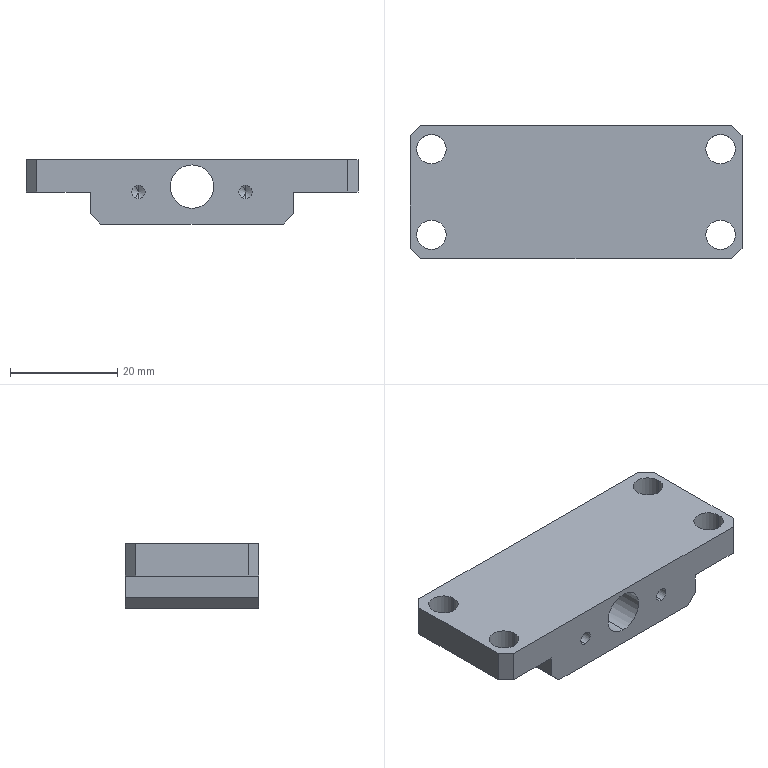Part | STEP file | 11-FG-SZ03111 | 1 solid | 38 faces | box 62 x 25 x 12 mm | volume 12866 mm3 | cylinder 18 | plane 16 | cone 4 | commonest cylinder face diameters 5.5 x8 2.5 x4 3.3 x4 8.1 x2
STEP:
#1=CARTESIAN_POINT('',(-29.75,8.,12.));
#2=VERTEX_POINT('',#1);
#3=CARTESIAN_POINT('',(-24.25,8.,12.));
#4=VERTEX_POINT('',#3);
#5=CARTESIAN_POINT('',(-27.,8.,12.));
#6=DIRECTION('',(0.,0.,1.));
#7=DIRECTION('',(1.,0.,0.));
#8=AXIS2_PLACEMENT_3D('',#5,#6,#7);
#9=CIRCLE('',#8,2.75);
#10=EDGE_CURVE('',#2,#4,#9,.T.);
#11=ORIENTED_EDGE('',*,*,#10,.T.);
#12=CARTESIAN_POINT('',(-24.25,8.,6.));
#13=VERTEX_POINT('',#12);
#14=CARTESIAN_POINT('',(-24.25,8.,24.));
#15=DIRECTION('',(0.,0.,-1.));
#16=VECTOR('',#15,1000.);
#17=LINE('',#14,#16);
#18=EDGE_CURVE('',#4,#13,#17,.T.);
#19=ORIENTED_EDGE('',*,*,#18,.T.);
#20=CARTESIAN_POINT('',(-29.75,8.,6.));
#21=VERTEX_POINT('',#20);
#22=CARTESIAN_POINT('',(-27.,8.,6.));
#23=DIRECTION('',(0.,0.,-1.));
#24=DIRECTION('',(-1.,0.,0.));
#25=AXIS2_PLACEMENT_3D('',#22,#23,#24);
#26=CIRCLE('',#25,2.75);
#27=EDGE_CURVE('',#13,#21,#26,.T.);
#28=ORIENTED_EDGE('',*,*,#27,.T.);
#29=CARTESIAN_POINT('',(-29.75,8.,24.));
#30=DIRECTION('',(0.,0.,-1.));
#31=VECTOR('',#30,1000.);
#32=LINE('',#29,#31);
#33=EDGE_CURVE('',#2,#21,#32,.T.);
#34=ORIENTED_EDGE('',*,*,#33,.F.);
#35=EDGE_LOOP('',(#11,#19,#28,#34));
#36=FACE_OUTER_BOUND('',#35,.T.);
#37=CARTESIAN_POINT('',(-27.,8.,24.));
#38=DIRECTION('',(0.,0.,-1.));
#39=DIRECTION('',(-1.,0.,0.));
#40=AXIS2_PLACEMENT_3D('',#37,#38,#39);
#41=CYLINDRICAL_SURFACE('',#40,2.75);
#42=ADVANCED_FACE('',(#36),#41,.F.);
#43=CARTESIAN_POINT('',(-29.75,-8.,12.));
#44=VERTEX_POINT('',#43);
#45=CARTESIAN_POINT('',(-24.25,-8.,12.));
#46=VERTEX_POINT('',#45);
#47=CARTESIAN_POINT('',(-27.,-8.,12.));
#48=DIRECTION('',(0.,0.,1.));
#49=DIRECTION('',(1.,0.,0.));
#50=AXIS2_PLACEMENT_3D('',#47,#48,#49);
#51=CIRCLE('',#50,2.75);
#52=EDGE_CURVE('',#44,#46,#51,.T.);
#53=ORIENTED_EDGE('',*,*,#52,.T.);
#54=CARTESIAN_POINT('',(-24.25,-8.,6.));
#55=VERTEX_POINT('',#54);
#56=CARTESIAN_POINT('',(-24.25,-8.,24.));
#57=DIRECTION('',(0.,0.,-1.));
#58=VECTOR('',#57,1000.);
#59=LINE('',#56,#58);
#60=EDGE_CURVE('',#46,#55,#59,.T.);
#61=ORIENTED_EDGE('',*,*,#60,.T.);
#62=CARTESIAN_POINT('',(-29.75,-8.,6.));
#63=VERTEX_POINT('',#62);
#64=CARTESIAN_POINT('',(-27.,-8.,6.));
#65=DIRECTION('',(0.,0.,-1.));
#66=DIRECTION('',(-1.,0.,0.));
#67=AXIS2_PLACEMENT_3D('',#64,#65,#66);
#68=CIRCLE('',#67,2.75);
#69=EDGE_CURVE('',#55,#63,#68,.T.);
#70=ORIENTED_EDGE('',*,*,#69,.T.);
#71=CARTESIAN_POINT('',(-29.75,-8.,24.));
#72=DIRECTION('',(0.,0.,-1.));
#73=VECTOR('',#72,1000.);
#74=LINE('',#71,#73);
#75=EDGE_CURVE('',#44,#63,#74,.T.);
#76=ORIENTED_EDGE('',*,*,#75,.F.);
#77=EDGE_LOOP('',(#53,#61,#70,#76));
#78=FACE_OUTER_BOUND('',#77,.T.);
#79=CARTESIAN_POINT('',(-27.,-8.,24.));
#80=DIRECTION('',(0.,0.,-1.));
#81=DIRECTION('',(-1.,0.,0.));
#82=AXIS2_PLACEMENT_3D('',#79,#80,#81);
#83=CYLINDRICAL_SURFACE('',#82,2.75);
#84=ADVANCED_FACE('',(#78),#83,.F.);
#85=CARTESIAN_POINT('',(24.25,-8.,12.));
#86=VERTEX_POINT('',#85);
#87=CARTESIAN_POINT('',(29.75,-8.,12.));
#88=VERTEX_POINT('',#87);
#89=CARTESIAN_POINT('',(27.,-8.,12.));
#90=DIRECTION('',(0.,0.,1.));
#91=DIRECTION('',(1.,0.,0.));
#92=AXIS2_PLACEMENT_3D('',#89,#90,#91);
#93=CIRCLE('',#92,2.75);
#94=EDGE_CURVE('',#86,#88,#93,.T.);
#95=ORIENTED_EDGE('',*,*,#94,.T.);
#96=CARTESIAN_POINT('',(29.75,-8.,6.));
#97=VERTEX_POINT('',#96);
#98=CARTESIAN_POINT('',(29.75,-8.,24.));
#99=DIRECTION('',(0.,0.,-1.));
#100=VECTOR('',#99,1000.);
#101=LINE('',#98,#100);
#102=EDGE_CURVE('',#88,#97,#101,.T.);
#103=ORIENTED_EDGE('',*,*,#102,.T.);
#104=CARTESIAN_POINT('',(24.25,-8.,6.));
#105=VERTEX_POINT('',#104);
#106=CARTESIAN_POINT('',(27.,-8.,6.));
#107=DIRECTION('',(0.,0.,-1.));
#108=DIRECTION('',(-1.,0.,0.));
#109=AXIS2_PLACEMENT_3D('',#106,#107,#108);
#110=CIRCLE('',#109,2.75);
#111=EDGE_CURVE('',#97,#105,#110,.T.);
#112=ORIENTED_EDGE('',*,*,#111,.T.);
#113=CARTESIAN_POINT('',(24.25,-8.,24.));
#114=DIRECTION('',(0.,0.,-1.));
#115=VECTOR('',#114,1000.);
#116=LINE('',#113,#115);
#117=EDGE_CURVE('',#86,#105,#116,.T.);
#118=ORIENTED_EDGE('',*,*,#117,.F.);
#119=EDGE_LOOP('',(#95,#103,#112,#118));
#120=FACE_OUTER_BOUND('',#119,.T.);
#121=CARTESIAN_POINT('',(27.,-8.,24.));
#122=DIRECTION('',(0.,0.,-1.));
#123=DIRECTION('',(-1.,0.,0.));
#124=AXIS2_PLACEMENT_3D('',#121,#122,#123);
#125=CYLINDRICAL_SURFACE('',#124,2.75);
#126=ADVANCED_FACE('',(#120),#125,.F.);
#127=CARTESIAN_POINT('',(24.25,8.,12.));
#128=VERTEX_POINT('',#127);
#129=CARTESIAN_POINT('',(29.75,8.,12.));
#130=VERTEX_POINT('',#129);
#131=CARTESIAN_POINT('',(27.,8.,12.));
#132=DIRECTION('',(0.,0.,1.));
#133=DIRECTION('',(1.,0.,0.));
#134=AXIS2_PLACEMENT_3D('',#131,#132,#133);
#135=CIRCLE('',#134,2.75);
#136=EDGE_CURVE('',#128,#130,#135,.T.);
#137=ORIENTED_EDGE('',*,*,#136,.T.);
#138=CARTESIAN_POINT('',(29.75,8.,6.));
#139=VERTEX_POINT('',#138);
#140=CARTESIAN_POINT('',(29.75,8.,24.));
#141=DIRECTION('',(0.,0.,-1.));
#142=VECTOR('',#141,1000.);
#143=LINE('',#140,#142);
#144=EDGE_CURVE('',#130,#139,#143,.T.);
#145=ORIENTED_EDGE('',*,*,#144,.T.);
#146=CARTESIAN_POINT('',(24.25,8.,6.));
#147=VERTEX_POINT('',#146);
#148=CARTESIAN_POINT('',(27.,8.,6.));
#149=DIRECTION('',(0.,0.,-1.));
#150=DIRECTION('',(-1.,0.,0.));
#151=AXIS2_PLACEMENT_3D('',#148,#149,#150);
#152=CIRCLE('',#151,2.75);
#153=EDGE_CURVE('',#139,#147,#152,.T.);
#154=ORIENTED_EDGE('',*,*,#153,.T.);
#155=CARTESIAN_POINT('',(24.25,8.,24.));
#156=DIRECTION('',(0.,0.,-1.));
#157=VECTOR('',#156,1000.);
#158=LINE('',#155,#157);
#159=EDGE_CURVE('',#128,#147,#158,.T.);
#160=ORIENTED_EDGE('',*,*,#159,.F.);
#161=EDGE_LOOP('',(#137,#145,#154,#160));
#162=FACE_OUTER_BOUND('',#161,.T.);
#163=CARTESIAN_POINT('',(27.,8.,24.));
#164=DIRECTION('',(0.,0.,-1.));
#165=DIRECTION('',(-1.,0.,0.));
#166=AXIS2_PLACEMENT_3D('',#163,#164,#165);
#167=CYLINDRICAL_SURFACE('',#166,2.75);
#168=ADVANCED_FACE('',(#162),#167,.F.);
#169=CARTESIAN_POINT('',(10.,-5.,7.25));
#170=VERTEX_POINT('',#169);
#171=CARTESIAN_POINT('',(10.,-5.,4.75));
#172=VERTEX_POINT('',#171);
#173=CARTESIAN_POINT('',(10.,-5.,6.));
#174=DIRECTION('',(0.,-1.,0.));
#175=DIRECTION('',(0.,0.,-1.));
#176=AXIS2_PLACEMENT_3D('',#173,#174,#175);
#177=CIRCLE('',#176,1.25);
#178=EDGE_CURVE('',#170,#172,#177,.T.);
#179=ORIENTED_EDGE('',*,*,#178,.F.);
#180=CARTESIAN_POINT('',(10.,-12.5,7.25));
#181=VERTEX_POINT('',#180);
#182=CARTESIAN_POINT('',(10.,-12.5,7.25));
#183=DIRECTION('',(0.,-1.,0.));
#184=VECTOR('',#183,1000.);
#185=LINE('',#182,#184);
#186=EDGE_CURVE('',#170,#181,#185,.T.);
#187=ORIENTED_EDGE('',*,*,#186,.T.);
#188=CARTESIAN_POINT('',(10.,-12.5,4.75));
#189=VERTEX_POINT('',#188);
#190=CARTESIAN_POINT('',(10.,-12.5,6.));
#191=DIRECTION('',(0.,-1.,0.));
#192=DIRECTION('',(0.,0.,-1.));
#193=AXIS2_PLACEMENT_3D('',#190,#191,#192);
#194=CIRCLE('',#193,1.25);
#195=EDGE_CURVE('',#181,#189,#194,.T.);
#196=ORIENTED_EDGE('',*,*,#195,.T.);
#197=CARTESIAN_POINT('',(10.,-12.5,4.75));
#198=DIRECTION('',(0.,-1.,0.));
#199=VECTOR('',#198,1000.);
#200=LINE('',#197,#199);
#201=EDGE_CURVE('',#172,#189,#200,.T.);
#202=ORIENTED_EDGE('',*,*,#201,.F.);
#203=EDGE_LOOP('',(#179,#187,#196,#202));
#204=FACE_OUTER_BOUND('',#203,.T.);
#205=CARTESIAN_POINT('',(10.,-12.5,6.));
#206=DIRECTION('',(0.,-1.,0.));
#207=DIRECTION('',(0.,0.,-1.));
#208=AXIS2_PLACEMENT_3D('',#205,#206,#207);
#209=CYLINDRICAL_SURFACE('',#208,1.25);
#210=ADVANCED_FACE('',(#204),#209,.F.);
#211=CARTESIAN_POINT('',(10.,-4.249,6.));
#212=VERTEX_POINT('',#211);
#213=CARTESIAN_POINT('',(10.,-5.,4.75));
#214=DIRECTION('',(0.,-0.515,-0.8572));
#215=VECTOR('',#214,1000.);
#216=LINE('',#213,#215);
#217=EDGE_CURVE('',#212,#172,#216,.T.);
#218=ORIENTED_EDGE('',*,*,#217,.F.);
#219=CARTESIAN_POINT('',(10.,-5.,7.25));
#220=DIRECTION('',(0.,-0.515,0.8572));
#221=VECTOR('',#220,1000.);
#222=LINE('',#219,#221);
#223=EDGE_CURVE('',#212,#170,#222,.T.);
#224=ORIENTED_EDGE('',*,*,#223,.T.);
#225=ORIENTED_EDGE('',*,*,#178,.T.);
#226=EDGE_LOOP('',(#218,#224,#225));
#227=FACE_OUTER_BOUND('',#226,.T.);
#228=CARTESIAN_POINT('',(10.,-5.,6.));
#229=DIRECTION('',(0.,-1.,0.));
#230=DIRECTION('',(0.,0.,-1.));
#231=AXIS2_PLACEMENT_3D('',#228,#229,#230);
#232=CONICAL_SURFACE('',#231,1.25,1.03);
#233=ADVANCED_FACE('',(#227),#232,.F.);
#234=CARTESIAN_POINT('',(-10.,-5.,7.25));
#235=VERTEX_POINT('',#234);
#236=CARTESIAN_POINT('',(-10.,-5.,4.75));
#237=VERTEX_POINT('',#236);
#238=CARTESIAN_POINT('',(-10.,-5.,6.));
#239=DIRECTION('',(0.,-1.,0.));
#240=DIRECTION('',(0.,0.,-1.));
#241=AXIS2_PLACEMENT_3D('',#238,#239,#240);
#242=CIRCLE('',#241,1.25);
#243=EDGE_CURVE('',#235,#237,#242,.T.);
#244=ORIENTED_EDGE('',*,*,#243,.F.);
#245=CARTESIAN_POINT('',(-10.,-12.5,7.25));
#246=VERTEX_POINT('',#245);
#247=CARTESIAN_POINT('',(-10.,-12.5,7.25));
#248=DIRECTION('',(0.,-1.,0.));
#249=VECTOR('',#248,1000.);
#250=LINE('',#247,#249);
#251=EDGE_CURVE('',#235,#246,#250,.T.);
#252=ORIENTED_EDGE('',*,*,#251,.T.);
#253=CARTESIAN_POINT('',(-10.,-12.5,4.75));
#254=VERTEX_POINT('',#253);
#255=CARTESIAN_POINT('',(-10.,-12.5,6.));
#256=DIRECTION('',(0.,-1.,0.));
#257=DIRECTION('',(0.,0.,-1.));
#258=AXIS2_PLACEMENT_3D('',#255,#256,#257);
#259=CIRCLE('',#258,1.25);
#260=EDGE_CURVE('',#246,#254,#259,.T.);
#261=ORIENTED_EDGE('',*,*,#260,.T.);
#262=CARTESIAN_POINT('',(-10.,-12.5,4.75));
#263=DIRECTION('',(0.,-1.,0.));
#264=VECTOR('',#263,1000.);
#265=LINE('',#262,#264);
#266=EDGE_CURVE('',#237,#254,#265,.T.);
#267=ORIENTED_EDGE('',*,*,#266,.F.);
#268=EDGE_LOOP('',(#244,#252,#261,#267));
#269=FACE_OUTER_BOUND('',#268,.T.);
#270=CARTESIAN_POINT('',(-10.,-12.5,6.));
#271=DIRECTION('',(0.,-1.,0.));
#272=DIRECTION('',(0.,0.,-1.));
#273=AXIS2_PLACEMENT_3D('',#270,#271,#272);
#274=CYLINDRICAL_SURFACE('',#273,1.25);
#275=ADVANCED_FACE('',(#269),#274,.F.);
#276=CARTESIAN_POINT('',(-10.,-4.249,6.));
#277=VERTEX_POINT('',#276);
#278=CARTESIAN_POINT('',(-10.,-5.,4.75));
#279=DIRECTION('',(0.,-0.515,-0.8572));
#280=VECTOR('',#279,1000.);
#281=LINE('',#278,#280);
#282=EDGE_CURVE('',#277,#237,#281,.T.);
#283=ORIENTED_EDGE('',*,*,#282,.F.);
#284=CARTESIAN_POINT('',(-10.,-5.,7.25));
#285=DIRECTION('',(0.,-0.515,0.8572));
#286=VECTOR('',#285,1000.);
#287=LINE('',#284,#286);
#288=EDGE_CURVE('',#277,#235,#287,.T.);
#289=ORIENTED_EDGE('',*,*,#288,.T.);
#290=ORIENTED_EDGE('',*,*,#243,.T.);
#291=EDGE_LOOP('',(#283,#289,#290));
#292=FACE_OUTER_BOUND('',#291,.T.);
#293=CARTESIAN_POINT('',(-10.,-5.,6.));
#294=DIRECTION('',(0.,-1.,0.));
#295=DIRECTION('',(0.,0.,-1.));
#296=AXIS2_PLACEMENT_3D('',#293,#294,#295);
#297=CONICAL_SURFACE('',#296,1.25,1.03);
#298=ADVANCED_FACE('',(#292),#297,.F.);
#299=CARTESIAN_POINT('',(1.65,6.,3.301));
#300=VERTEX_POINT('',#299);
#301=CARTESIAN_POINT('',(0.,4.35,2.95));
#302=VERTEX_POINT('',#301);
#303=CARTESIAN_POINT('',(1.65,6.,3.301));
#304=CARTESIAN_POINT('',(1.65,5.891,3.301));
#305=CARTESIAN_POINT('',(1.639,5.78,3.296));
#306=CARTESIAN_POINT('',(1.596,5.568,3.278));
#307=CARTESIAN_POINT('',(1.564,5.464,3.264));
#308=CARTESIAN_POINT('',(1.48,5.263,3.23));
#309=CARTESIAN_POINT('',(1.43,5.169,3.21));
#310=CARTESIAN_POINT('',(1.31,4.992,3.167));
#311=CARTESIAN_POINT('',(1.241,4.908,3.144));
#312=CARTESIAN_POINT('',(1.09,4.757,3.099));
#313=CARTESIAN_POINT('',(1.008,4.69,3.076));
#314=CARTESIAN_POINT('',(0.83,4.57,3.035));
#315=CARTESIAN_POINT('',(0.734,4.518,3.016));
#316=CARTESIAN_POINT('',(0.4366,4.394,2.969));
#317=CARTESIAN_POINT('',(0.2172,4.35,2.95));
#318=CARTESIAN_POINT('',(0.,4.35,2.95));
#319=B_SPLINE_CURVE_WITH_KNOTS('',3,(#303,#304,#305,#306,#307,#308,#309,#310,#311,#312,#313,#314,#315,#316,#317,#318),.UNSPECIFIED.,.F.,.F.,(4,2,2,2,2,2,2,4),(0.002609,0.002935,0.003261,0.003587,0.003913,0.004238,0.004564,0.005216),.UNSPECIFIED.);
#320=EDGE_CURVE('',#300,#302,#319,.T.);
#321=ORIENTED_EDGE('',*,*,#320,.F.);
#322=CARTESIAN_POINT('',(1.65,6.,0.));
#323=VERTEX_POINT('',#322);
#324=CARTESIAN_POINT('',(1.65,6.,0.));
#325=DIRECTION('',(0.,0.,-1.));
#326=VECTOR('',#325,1000.);
#327=LINE('',#324,#326);
#328=EDGE_CURVE('',#300,#323,#327,.T.);
#329=ORIENTED_EDGE('',*,*,#328,.T.);
#330=CARTESIAN_POINT('',(-1.65,6.,0.));
#331=VERTEX_POINT('',#330);
#332=CARTESIAN_POINT('',(0.,6.,0.));
#333=DIRECTION('',(0.,0.,-1.));
#334=DIRECTION('',(-1.,0.,0.));
#335=AXIS2_PLACEMENT_3D('',#332,#333,#334);
#336=CIRCLE('',#335,1.65);
#337=EDGE_CURVE('',#323,#331,#336,.T.);
#338=ORIENTED_EDGE('',*,*,#337,.T.);
#339=CARTESIAN_POINT('',(-1.65,6.,3.301));
#340=VERTEX_POINT('',#339);
#341=CARTESIAN_POINT('',(-1.65,6.,0.));
#342=DIRECTION('',(0.,0.,-1.));
#343=VECTOR('',#342,1000.);
#344=LINE('',#341,#343);
#345=EDGE_CURVE('',#340,#331,#344,.T.);
#346=ORIENTED_EDGE('',*,*,#345,.F.);
#347=CARTESIAN_POINT('',(0.,4.35,2.95));
#348=CARTESIAN_POINT('',(-0.1086,4.35,2.95));
#349=CARTESIAN_POINT('',(-0.2187,4.361,2.954));
#350=CARTESIAN_POINT('',(-0.4326,4.404,2.972));
#351=CARTESIAN_POINT('',(-0.5359,4.436,2.984));
#352=CARTESIAN_POINT('',(-0.8354,4.561,3.032));
#353=CARTESIAN_POINT('',(-1.016,4.682,3.076));
#354=CARTESIAN_POINT('',(-1.244,4.91,3.145));
#355=CARTESIAN_POINT('',(-1.311,4.993,3.168));
#356=CARTESIAN_POINT('',(-1.43,5.17,3.21));
#357=CARTESIAN_POINT('',(-1.482,5.266,3.23));
#358=CARTESIAN_POINT('',(-1.565,5.465,3.264));
#359=CARTESIAN_POINT('',(-1.596,5.568,3.278));
#360=CARTESIAN_POINT('',(-1.639,5.781,3.296));
#361=CARTESIAN_POINT('',(-1.65,5.891,3.301));
#362=CARTESIAN_POINT('',(-1.65,6.,3.301));
#363=B_SPLINE_CURVE_WITH_KNOTS('',3,(#347,#348,#349,#350,#351,#352,#353,#354,#355,#356,#357,#358,#359,#360,#361,#362),.UNSPECIFIED.,.F.,.F.,(4,2,2,2,2,2,2,4),(0.005216,0.005542,0.005868,0.006519,0.006845,0.007171,0.007497,0.007822),.UNSPECIFIED.);
#364=EDGE_CURVE('',#302,#340,#363,.T.);
#365=ORIENTED_EDGE('',*,*,#364,.F.);
#366=EDGE_LOOP('',(#321,#329,#338,#346,#365));
#367=FACE_OUTER_BOUND('',#366,.T.);
#368=CARTESIAN_POINT('',(0.,6.,0.));
#369=DIRECTION('',(0.,0.,-1.));
#370=DIRECTION('',(-1.,0.,0.));
#371=AXIS2_PLACEMENT_3D('',#368,#369,#370);
#372=CYLINDRICAL_SURFACE('',#371,1.65);
#373=ADVANCED_FACE('',(#367),#372,.F.);
#374=CARTESIAN_POINT('',(1.65,-6.,3.301));
#375=VERTEX_POINT('',#374);
#376=CARTESIAN_POINT('',(0.,-7.65,2.95));
#377=VERTEX_POINT('',#376);
#378=CARTESIAN_POINT('',(1.65,-6.,3.301));
#379=CARTESIAN_POINT('',(1.65,-6.109,3.301));
#380=CARTESIAN_POINT('',(1.639,-6.22,3.296));
#381=CARTESIAN_POINT('',(1.596,-6.432,3.278));
#382=CARTESIAN_POINT('',(1.564,-6.536,3.264));
#383=CARTESIAN_POINT('',(1.48,-6.737,3.23));
#384=CARTESIAN_POINT('',(1.43,-6.831,3.21));
#385=CARTESIAN_POINT('',(1.31,-7.008,3.167));
#386=CARTESIAN_POINT('',(1.241,-7.092,3.144));
#387=CARTESIAN_POINT('',(1.09,-7.243,3.099));
#388=CARTESIAN_POINT('',(1.008,-7.31,3.076));
#389=CARTESIAN_POINT('',(0.83,-7.43,3.035));
#390=CARTESIAN_POINT('',(0.734,-7.482,3.016));
#391=CARTESIAN_POINT('',(0.4366,-7.606,2.969));
#392=CARTESIAN_POINT('',(0.2172,-7.65,2.95));
#393=CARTESIAN_POINT('',(0.,-7.65,2.95));
#394=B_SPLINE_CURVE_WITH_KNOTS('',3,(#378,#379,#380,#381,#382,#383,#384,#385,#386,#387,#388,#389,#390,#391,#392,#393),.UNSPECIFIED.,.F.,.F.,(4,2,2,2,2,2,2,4),(0.002609,0.002935,0.003261,0.003587,0.003913,0.004238,0.004564,0.005216),.UNSPECIFIED.);
#395=EDGE_CURVE('',#375,#377,#394,.T.);
#396=ORIENTED_EDGE('',*,*,#395,.F.);
#397=CARTESIAN_POINT('',(1.65,-6.,0.));
#398=VERTEX_POINT('',#397);
#399=CARTESIAN_POINT('',(1.65,-6.,0.));
#400=DIRECTION('',(0.,0.,-1.));
#401=VECTOR('',#400,1000.);
#402=LINE('',#399,#401);
#403=EDGE_CURVE('',#375,#398,#402,.T.);
#404=ORIENTED_EDGE('',*,*,#403,.T.);
#405=CARTESIAN_POINT('',(-1.65,-6.,0.));
#406=VERTEX_POINT('',#405);
#407=CARTESIAN_POINT('',(0.,-6.,0.));
#408=DIRECTION('',(0.,0.,-1.));
#409=DIRECTION('',(-1.,0.,0.));
#410=AXIS2_PLACEMENT_3D('',#407,#408,#409);
#411=CIRCLE('',#410,1.65);
#412=EDGE_CURVE('',#398,#406,#411,.T.);
#413=ORIENTED_EDGE('',*,*,#412,.T.);
#414=CARTESIAN_POINT('',(-1.65,-6.,3.301));
#415=VERTEX_POINT('',#414);
#416=CARTESIAN_POINT('',(-1.65,-6.,0.));
#417=DIRECTION('',(0.,0.,-1.));
#418=VECTOR('',#417,1000.);
#419=LINE('',#416,#418);
#420=EDGE_CURVE('',#415,#406,#419,.T.);
#421=ORIENTED_EDGE('',*,*,#420,.F.);
#422=CARTESIAN_POINT('',(0.,-7.65,2.95));
#423=CARTESIAN_POINT('',(-0.1086,-7.65,2.95));
#424=CARTESIAN_POINT('',(-0.2187,-7.639,2.954));
#425=CARTESIAN_POINT('',(-0.4326,-7.596,2.972));
#426=CARTESIAN_POINT('',(-0.5359,-7.564,2.984));
#427=CARTESIAN_POINT('',(-0.8354,-7.439,3.032));
#428=CARTESIAN_POINT('',(-1.016,-7.318,3.076));
#429=CARTESIAN_POINT('',(-1.244,-7.09,3.145));
#430=CARTESIAN_POINT('',(-1.311,-7.007,3.168));
#431=CARTESIAN_POINT('',(-1.43,-6.83,3.21));
#432=CARTESIAN_POINT('',(-1.482,-6.734,3.23));
#433=CARTESIAN_POINT('',(-1.565,-6.535,3.264));
#434=CARTESIAN_POINT('',(-1.596,-6.432,3.278));
#435=CARTESIAN_POINT('',(-1.639,-6.219,3.296));
#436=CARTESIAN_POINT('',(-1.65,-6.109,3.301));
#437=CARTESIAN_POINT('',(-1.65,-6.,3.301));
#438=B_SPLINE_CURVE_WITH_KNOTS('',3,(#422,#423,#424,#425,#426,#427,#428,#429,#430,#431,#432,#433,#434,#435,#436,#437),.UNSPECIFIED.,.F.,.F.,(4,2,2,2,2,2,2,4),(0.005216,0.005542,0.005868,0.006519,0.006845,0.007171,0.007497,0.007822),.UNSPECIFIED.);
#439=EDGE_CURVE('',#377,#415,#438,.T.);
#440=ORIENTED_EDGE('',*,*,#439,.F.);
#441=EDGE_LOOP('',(#396,#404,#413,#421,#440));
#442=FACE_OUTER_BOUND('',#441,.T.);
#443=CARTESIAN_POINT('',(0.,-6.,0.));
#444=DIRECTION('',(0.,0.,-1.));
#445=DIRECTION('',(-1.,0.,0.));
#446=AXIS2_PLACEMENT_3D('',#443,#444,#445);
#447=CYLINDRICAL_SURFACE('',#446,1.65);
#448=ADVANCED_FACE('',(#442),#447,.F.);
#449=CARTESIAN_POINT('',(0.,12.5,11.05));
#450=VERTEX_POINT('',#449);
#451=CARTESIAN_POINT('',(0.,12.5,2.95));
#452=VERTEX_POINT('',#451);
#453=CARTESIAN_POINT('',(0.,12.5,7.));
#454=DIRECTION('',(0.,-1.,0.));
#455=DIRECTION('',(0.,0.,-1.));
#456=AXIS2_PLACEMENT_3D('',#453,#454,#455);
#457=CIRCLE('',#456,4.05);
#458=EDGE_CURVE('',#450,#452,#457,.T.);
#459=ORIENTED_EDGE('',*,*,#458,.F.);
#460=CARTESIAN_POINT('',(0.,-12.5,11.05));
#461=VERTEX_POINT('',#460);
#462=CARTESIAN_POINT('',(0.,12.5,11.05));
#463=DIRECTION('',(0.,-1.,0.));
#464=VECTOR('',#463,1000.);
#465=LINE('',#462,#464);
#466=EDGE_CURVE('',#450,#461,#465,.T.);
#467=ORIENTED_EDGE('',*,*,#466,.T.);
#468=CARTESIAN_POINT('',(0.,-12.5,2.95));
#469=VERTEX_POINT('',#468);
#470=CARTESIAN_POINT('',(0.,-12.5,7.));
#471=DIRECTION('',(0.,-1.,0.));
#472=DIRECTION('',(0.,0.,-1.));
#473=AXIS2_PLACEMENT_3D('',#470,#471,#472);
#474=CIRCLE('',#473,4.05);
#475=EDGE_CURVE('',#461,#469,#474,.T.);
#476=ORIENTED_EDGE('',*,*,#475,.T.);
#477=CARTESIAN_POINT('',(0.,12.5,2.95));
#478=DIRECTION('',(0.,-1.,0.));
#479=VECTOR('',#478,1000.);
#480=LINE('',#477,#479);
#481=EDGE_CURVE('',#377,#469,#480,.T.);
#482=ORIENTED_EDGE('',*,*,#481,.F.);
#483=ORIENTED_EDGE('',*,*,#439,.T.);
#484=CARTESIAN_POINT('',(0.,-4.35,2.95));
#485=VERTEX_POINT('',#484);
#486=CARTESIAN_POINT('',(-1.65,-6.,3.301));
#487=CARTESIAN_POINT('',(-1.65,-5.783,3.301));
#488=CARTESIAN_POINT('',(-1.606,-5.564,3.281));
#489=CARTESIAN_POINT('',(-1.481,-5.266,3.23));
#490=CARTESIAN_POINT('',(-1.43,-5.17,3.21));
#491=CARTESIAN_POINT('',(-1.31,-4.992,3.167));
#492=CARTESIAN_POINT('',(-1.243,-4.909,3.145));
#493=CARTESIAN_POINT('',(-1.092,-4.758,3.099));
#494=CARTESIAN_POINT('',(-1.008,-4.689,3.076));
#495=CARTESIAN_POINT('',(-0.8309,-4.57,3.035));
#496=CARTESIAN_POINT('',(-0.7366,-4.52,3.016));
#497=CARTESIAN_POINT('',(-0.4349,-4.393,2.968));
#498=CARTESIAN_POINT('',(-0.2204,-4.35,2.95));
#499=CARTESIAN_POINT('',(0.,-4.35,2.95));
#500=B_SPLINE_CURVE_WITH_KNOTS('',3,(#486,#487,#488,#489,#490,#491,#492,#493,#494,#495,#496,#497,#498,#499),.UNSPECIFIED.,.F.,.F.,(4,2,2,2,2,2,4),(0.007822,0.008474,0.0088,0.009125,0.009451,0.009777,0.01043),.UNSPECIFIED.);
#501=EDGE_CURVE('',#415,#485,#500,.T.);
#502=ORIENTED_EDGE('',*,*,#501,.T.);
#503=CARTESIAN_POINT('',(0.,12.5,2.95));
#504=DIRECTION('',(0.,-1.,0.));
#505=VECTOR('',#504,1000.);
#506=LINE('',#503,#505);
#507=EDGE_CURVE('',#302,#485,#506,.T.);
#508=ORIENTED_EDGE('',*,*,#507,.F.);
#509=ORIENTED_EDGE('',*,*,#364,.T.);
#510=CARTESIAN_POINT('',(0.,7.65,2.95));
#511=VERTEX_POINT('',#510);
#512=CARTESIAN_POINT('',(-1.65,6.,3.301));
#513=CARTESIAN_POINT('',(-1.65,6.217,3.301));
#514=CARTESIAN_POINT('',(-1.606,6.436,3.281));
#515=CARTESIAN_POINT('',(-1.481,6.734,3.23));
#516=CARTESIAN_POINT('',(-1.43,6.83,3.21));
#517=CARTESIAN_POINT('',(-1.31,7.008,3.167));
#518=CARTESIAN_POINT('',(-1.243,7.091,3.145));
#519=CARTESIAN_POINT('',(-1.092,7.242,3.099));
#520=CARTESIAN_POINT('',(-1.008,7.311,3.076));
#521=CARTESIAN_POINT('',(-0.8309,7.43,3.035));
#522=CARTESIAN_POINT('',(-0.7366,7.48,3.016));
#523=CARTESIAN_POINT('',(-0.4349,7.607,2.968));
#524=CARTESIAN_POINT('',(-0.2204,7.65,2.95));
#525=CARTESIAN_POINT('',(0.,7.65,2.95));
#526=B_SPLINE_CURVE_WITH_KNOTS('',3,(#512,#513,#514,#515,#516,#517,#518,#519,#520,#521,#522,#523,#524,#525),.UNSPECIFIED.,.F.,.F.,(4,2,2,2,2,2,4),(0.007822,0.008474,0.0088,0.009125,0.009451,0.009777,0.01043),.UNSPECIFIED.);
#527=EDGE_CURVE('',#340,#511,#526,.T.);
#528=ORIENTED_EDGE('',*,*,#527,.T.);
#529=CARTESIAN_POINT('',(0.,12.5,2.95));
#530=DIRECTION('',(0.,-1.,0.));
#531=VECTOR('',#530,1000.);
#532=LINE('',#529,#531);
#533=EDGE_CURVE('',#452,#511,#532,.T.);
#534=ORIENTED_EDGE('',*,*,#533,.F.);
#535=EDGE_LOOP('',(#459,#467,#476,#482,#483,#502,#508,#509,#528,#534));
#536=FACE_OUTER_BOUND('',#535,.T.);
#537=CARTESIAN_POINT('',(0.,12.5,7.));
#538=DIRECTION('',(0.,-1.,0.));
#539=DIRECTION('',(0.,0.,-1.));
#540=AXIS2_PLACEMENT_3D('',#537,#538,#539);
#541=CYLINDRICAL_SURFACE('',#540,4.05);
#542=ADVANCED_FACE('',(#536),#541,.F.);
#543=CARTESIAN_POINT('',(31.,-10.5,6.));
#544=VERTEX_POINT('',#543);
#545=CARTESIAN_POINT('',(31.,10.5,6.));
#546=VERTEX_POINT('',#545);
#547=CARTESIAN_POINT('',(31.,-12.5,6.));
#548=DIRECTION('',(0.,1.,0.));
#549=VECTOR('',#548,1000.);
#550=LINE('',#547,#549);
#551=EDGE_CURVE('',#544,#546,#550,.T.);
#552=ORIENTED_EDGE('',*,*,#551,.T.);
#553=CARTESIAN_POINT('',(31.,10.5,12.));
#554=VERTEX_POINT('',#553);
#555=CARTESIAN_POINT('',(31.,10.5,12.));
#556=DIRECTION('',(0.,0.,1.));
#557=VECTOR('',#556,1000.);
#558=LINE('',#555,#557);
#559=EDGE_CURVE('',#546,#554,#558,.T.);
#560=ORIENTED_EDGE('',*,*,#559,.T.);
#561=CARTESIAN_POINT('',(31.,-10.5,12.));
#562=VERTEX_POINT('',#561);
#563=CARTESIAN_POINT('',(31.,12.5,12.));
#564=DIRECTION('',(0.,1.,0.));
#565=VECTOR('',#564,1000.);
#566=LINE('',#563,#565);
#567=EDGE_CURVE('',#562,#554,#566,.T.);
#568=ORIENTED_EDGE('',*,*,#567,.F.);
#569=CARTESIAN_POINT('',(31.,-10.5,12.));
#570=DIRECTION('',(0.,0.,-1.));
#571=VECTOR('',#570,1000.);
#572=LINE('',#569,#571);
#573=EDGE_CURVE('',#562,#544,#572,.T.);
#574=ORIENTED_EDGE('',*,*,#573,.T.);
#575=EDGE_LOOP('',(#552,#560,#568,#574));
#576=FACE_OUTER_BOUND('',#575,.T.);
#577=CARTESIAN_POINT('',(31.,12.5,12.));
#578=DIRECTION('',(-1.,0.,0.));
#579=DIRECTION('',(0.,-1.,0.));
#580=AXIS2_PLACEMENT_3D('',#577,#578,#579);
#581=PLANE('',#580);
#582=ADVANCED_FACE('',(#576),#581,.F.);
#583=CARTESIAN_POINT('',(0.,12.5,7.));
#584=DIRECTION('',(0.,-1.,0.));
#585=DIRECTION('',(0.,0.,-1.));
#586=AXIS2_PLACEMENT_3D('',#583,#584,#585);
#587=CIRCLE('',#586,4.05);
#588=EDGE_CURVE('',#452,#450,#587,.T.);
#589=ORIENTED_EDGE('',*,*,#588,.T.);
#590=ORIENTED_EDGE('',*,*,#458,.T.);
#591=EDGE_LOOP('',(#589,#590));
#592=FACE_BOUND('',#591,.T.);
#593=CARTESIAN_POINT('',(17.,12.5,0.));
#594=VERTEX_POINT('',#593);
#595=CARTESIAN_POINT('',(-17.,12.5,0.));
#596=VERTEX_POINT('',#595);
#597=CARTESIAN_POINT('',(-31.,12.5,0.));
#598=DIRECTION('',(-1.,0.,0.));
#599=VECTOR('',#598,1000.);
#600=LINE('',#597,#599);
#601=EDGE_CURVE('',#594,#596,#600,.T.);
#602=ORIENTED_EDGE('',*,*,#601,.T.);
#603=CARTESIAN_POINT('',(-19.,12.5,2.));
#604=VERTEX_POINT('',#603);
#605=CARTESIAN_POINT('',(-17.,12.5,0.));
#606=DIRECTION('',(-0.7071,0.,0.7071));
#607=VECTOR('',#606,1000.);
#608=LINE('',#605,#607);
#609=EDGE_CURVE('',#596,#604,#608,.T.);
#610=ORIENTED_EDGE('',*,*,#609,.T.);
#611=CARTESIAN_POINT('',(-19.,12.5,6.));
#612=VERTEX_POINT('',#611);
#613=CARTESIAN_POINT('',(-19.,12.5,0.));
#614=DIRECTION('',(0.,0.,-1.));
#615=VECTOR('',#614,1000.);
#616=LINE('',#613,#615);
#617=EDGE_CURVE('',#612,#604,#616,.T.);
#618=ORIENTED_EDGE('',*,*,#617,.F.);
#619=CARTESIAN_POINT('',(-29.,12.5,6.));
#620=VERTEX_POINT('',#619);
#621=CARTESIAN_POINT('',(-31.,12.5,6.));
#622=DIRECTION('',(1.,0.,0.));
#623=VECTOR('',#622,1000.);
#624=LINE('',#621,#623);
#625=EDGE_CURVE('',#620,#612,#624,.T.);
#626=ORIENTED_EDGE('',*,*,#625,.F.);
#627=CARTESIAN_POINT('',(-29.,12.5,12.));
#628=VERTEX_POINT('',#627);
#629=CARTESIAN_POINT('',(-29.,12.5,12.));
#630=DIRECTION('',(0.,0.,1.));
#631=VECTOR('',#630,1000.);
#632=LINE('',#629,#631);
#633=EDGE_CURVE('',#620,#628,#632,.T.);
#634=ORIENTED_EDGE('',*,*,#633,.T.);
#635=CARTESIAN_POINT('',(29.,12.5,12.));
#636=VERTEX_POINT('',#635);
#637=CARTESIAN_POINT('',(-31.,12.5,12.));
#638=DIRECTION('',(-1.,0.,0.));
#639=VECTOR('',#638,1000.);
#640=LINE('',#637,#639);
#641=EDGE_CURVE('',#636,#628,#640,.T.);
#642=ORIENTED_EDGE('',*,*,#641,.F.);
#643=CARTESIAN_POINT('',(29.,12.5,6.));
#644=VERTEX_POINT('',#643);
#645=CARTESIAN_POINT('',(29.,12.5,12.));
#646=DIRECTION('',(0.,0.,-1.));
#647=VECTOR('',#646,1000.);
#648=LINE('',#645,#647);
#649=EDGE_CURVE('',#636,#644,#648,.T.);
#650=ORIENTED_EDGE('',*,*,#649,.T.);
#651=CARTESIAN_POINT('',(19.,12.5,6.));
#652=VERTEX_POINT('',#651);
#653=CARTESIAN_POINT('',(31.,12.5,6.));
#654=DIRECTION('',(1.,0.,0.));
#655=VECTOR('',#654,1000.);
#656=LINE('',#653,#655);
#657=EDGE_CURVE('',#652,#644,#656,.T.);
#658=ORIENTED_EDGE('',*,*,#657,.F.);
#659=CARTESIAN_POINT('',(19.,12.5,2.));
#660=VERTEX_POINT('',#659);
#661=CARTESIAN_POINT('',(19.,12.5,0.));
#662=DIRECTION('',(0.,0.,1.));
#663=VECTOR('',#662,1000.);
#664=LINE('',#661,#663);
#665=EDGE_CURVE('',#660,#652,#664,.T.);
#666=ORIENTED_EDGE('',*,*,#665,.F.);
#667=CARTESIAN_POINT('',(19.,12.5,2.));
#668=DIRECTION('',(-0.7071,0.,-0.7071));
#669=VECTOR('',#668,1000.);
#670=LINE('',#667,#669);
#671=EDGE_CURVE('',#660,#594,#670,.T.);
#672=ORIENTED_EDGE('',*,*,#671,.T.);
#673=EDGE_LOOP('',(#602,#610,#618,#626,#634,#642,#650,#658,#666,#672));
#674=FACE_OUTER_BOUND('',#673,.T.);
#675=CARTESIAN_POINT('',(-31.,12.5,12.));
#676=DIRECTION('',(0.,-1.,0.));
#677=DIRECTION('',(0.,0.,-1.));
#678=AXIS2_PLACEMENT_3D('',#675,#676,#677);
#679=PLANE('',#678);
#680=ADVANCED_FACE('',(#592,#674),#679,.F.);
#681=CARTESIAN_POINT('',(-31.,10.5,12.));
#682=VERTEX_POINT('',#681);
#683=CARTESIAN_POINT('',(-31.,-10.5,12.));
#684=VERTEX_POINT('',#683);
#685=CARTESIAN_POINT('',(-31.,12.5,12.));
#686=DIRECTION('',(0.,-1.,0.));
#687=VECTOR('',#686,1000.);
#688=LINE('',#685,#687);
#689=EDGE_CURVE('',#682,#684,#688,.T.);
#690=ORIENTED_EDGE('',*,*,#689,.F.);
#691=CARTESIAN_POINT('',(-31.,10.5,6.));
#692=VERTEX_POINT('',#691);
#693=CARTESIAN_POINT('',(-31.,10.5,12.));
#694=DIRECTION('',(0.,0.,-1.));
#695=VECTOR('',#694,1000.);
#696=LINE('',#693,#695);
#697=EDGE_CURVE('',#682,#692,#696,.T.);
#698=ORIENTED_EDGE('',*,*,#697,.T.);
#699=CARTESIAN_POINT('',(-31.,-10.5,6.));
#700=VERTEX_POINT('',#699);
#701=CARTESIAN_POINT('',(-31.,-12.5,6.));
#702=DIRECTION('',(0.,1.,0.));
#703=VECTOR('',#702,1000.);
#704=LINE('',#701,#703);
#705=EDGE_CURVE('',#700,#692,#704,.T.);
#706=ORIENTED_EDGE('',*,*,#705,.F.);
#707=CARTESIAN_POINT('',(-31.,-10.5,12.));
#708=DIRECTION('',(0.,0.,1.));
#709=VECTOR('',#708,1000.);
#710=LINE('',#707,#709);
#711=EDGE_CURVE('',#700,#684,#710,.T.);
#712=ORIENTED_EDGE('',*,*,#711,.T.);
#713=EDGE_LOOP('',(#690,#698,#706,#712));
#714=FACE_OUTER_BOUND('',#713,.T.);
#715=CARTESIAN_POINT('',(-31.,12.5,12.));
#716=DIRECTION('',(1.,0.,0.));
#717=DIRECTION('',(0.,1.,0.));
#718=AXIS2_PLACEMENT_3D('',#715,#716,#717);
#719=PLANE('',#718);
#720=ADVANCED_FACE('',(#714),#719,.F.);
#721=CARTESIAN_POINT('',(10.,-12.5,6.));
#722=DIRECTION('',(0.,-1.,0.));
#723=DIRECTION('',(0.,0.,-1.));
#724=AXIS2_PLACEMENT_3D('',#721,#722,#723);
#725=CIRCLE('',#724,1.25);
#726=EDGE_CURVE('',#189,#181,#725,.T.);
#727=ORIENTED_EDGE('',*,*,#726,.F.);
#728=ORIENTED_EDGE('',*,*,#195,.F.);
#729=EDGE_LOOP('',(#727,#728));
#730=FACE_BOUND('',#729,.T.);
#731=CARTESIAN_POINT('',(-10.,-12.5,6.));
#732=DIRECTION('',(0.,-1.,0.));
#733=DIRECTION('',(0.,0.,-1.));
#734=AXIS2_PLACEMENT_3D('',#731,#732,#733);
#735=CIRCLE('',#734,1.25);
#736=EDGE_CURVE('',#254,#246,#735,.T.);
#737=ORIENTED_EDGE('',*,*,#736,.F.);
#738=ORIENTED_EDGE('',*,*,#260,.F.);
#739=EDGE_LOOP('',(#737,#738));
#740=FACE_BOUND('',#739,.T.);
#741=CARTESIAN_POINT('',(0.,-12.5,7.));
#742=DIRECTION('',(0.,-1.,0.));
#743=DIRECTION('',(0.,0.,-1.));
#744=AXIS2_PLACEMENT_3D('',#741,#742,#743);
#745=CIRCLE('',#744,4.05);
#746=EDGE_CURVE('',#469,#461,#745,.T.);
#747=ORIENTED_EDGE('',*,*,#746,.F.);
#748=ORIENTED_EDGE('',*,*,#475,.F.);
#749=EDGE_LOOP('',(#747,#748));
#750=FACE_BOUND('',#749,.T.);
#751=CARTESIAN_POINT('',(-19.,-12.5,6.));
#752=VERTEX_POINT('',#751);
#753=CARTESIAN_POINT('',(-19.,-12.5,2.));
#754=VERTEX_POINT('',#753);
#755=CARTESIAN_POINT('',(-19.,-12.5,0.));
#756=DIRECTION('',(0.,0.,-1.));
#757=VECTOR('',#756,1000.);
#758=LINE('',#755,#757);
#759=EDGE_CURVE('',#752,#754,#758,.T.);
#760=ORIENTED_EDGE('',*,*,#759,.T.);
#761=CARTESIAN_POINT('',(-17.,-12.5,0.));
#762=VERTEX_POINT('',#761);
#763=CARTESIAN_POINT('',(-17.,-12.5,0.));
#764=DIRECTION('',(0.7071,0.,-0.7071));
#765=VECTOR('',#764,1000.);
#766=LINE('',#763,#765);
#767=EDGE_CURVE('',#754,#762,#766,.T.);
#768=ORIENTED_EDGE('',*,*,#767,.T.);
#769=CARTESIAN_POINT('',(17.,-12.5,0.));
#770=VERTEX_POINT('',#769);
#771=CARTESIAN_POINT('',(-31.,-12.5,0.));
#772=DIRECTION('',(1.,0.,0.));
#773=VECTOR('',#772,1000.);
#774=LINE('',#771,#773);
#775=EDGE_CURVE('',#762,#770,#774,.T.);
#776=ORIENTED_EDGE('',*,*,#775,.T.);
#777=CARTESIAN_POINT('',(19.,-12.5,2.));
#778=VERTEX_POINT('',#777);
#779=CARTESIAN_POINT('',(19.,-12.5,2.));
#780=DIRECTION('',(0.7071,0.,0.7071));
#781=VECTOR('',#780,1000.);
#782=LINE('',#779,#781);
#783=EDGE_CURVE('',#770,#778,#782,.T.);
#784=ORIENTED_EDGE('',*,*,#783,.T.);
#785=CARTESIAN_POINT('',(19.,-12.5,6.));
#786=VERTEX_POINT('',#785);
#787=CARTESIAN_POINT('',(19.,-12.5,0.));
#788=DIRECTION('',(0.,0.,1.));
#789=VECTOR('',#788,1000.);
#790=LINE('',#787,#789);
#791=EDGE_CURVE('',#778,#786,#790,.T.);
#792=ORIENTED_EDGE('',*,*,#791,.T.);
#793=CARTESIAN_POINT('',(29.,-12.5,6.));
#794=VERTEX_POINT('',#793);
#795=CARTESIAN_POINT('',(31.,-12.5,6.));
#796=DIRECTION('',(1.,0.,0.));
#797=VECTOR('',#796,1000.);
#798=LINE('',#795,#797);
#799=EDGE_CURVE('',#786,#794,#798,.T.);
#800=ORIENTED_EDGE('',*,*,#799,.T.);
#801=CARTESIAN_POINT('',(29.,-12.5,12.));
#802=VERTEX_POINT('',#801);
#803=CARTESIAN_POINT('',(29.,-12.5,12.));
#804=DIRECTION('',(0.,0.,1.));
#805=VECTOR('',#804,1000.);
#806=LINE('',#803,#805);
#807=EDGE_CURVE('',#794,#802,#806,.T.);
#808=ORIENTED_EDGE('',*,*,#807,.T.);
#809=CARTESIAN_POINT('',(-29.,-12.5,12.));
#810=VERTEX_POINT('',#809);
#811=CARTESIAN_POINT('',(-31.,-12.5,12.));
#812=DIRECTION('',(1.,0.,0.));
#813=VECTOR('',#812,1000.);
#814=LINE('',#811,#813);
#815=EDGE_CURVE('',#810,#802,#814,.T.);
#816=ORIENTED_EDGE('',*,*,#815,.F.);
#817=CARTESIAN_POINT('',(-29.,-12.5,6.));
#818=VERTEX_POINT('',#817);
#819=CARTESIAN_POINT('',(-29.,-12.5,12.));
#820=DIRECTION('',(0.,0.,-1.));
#821=VECTOR('',#820,1000.);
#822=LINE('',#819,#821);
#823=EDGE_CURVE('',#810,#818,#822,.T.);
#824=ORIENTED_EDGE('',*,*,#823,.T.);
#825=CARTESIAN_POINT('',(-31.,-12.5,6.));
#826=DIRECTION('',(1.,0.,0.));
#827=VECTOR('',#826,1000.);
#828=LINE('',#825,#827);
#829=EDGE_CURVE('',#818,#752,#828,.T.);
#830=ORIENTED_EDGE('',*,*,#829,.T.);
#831=EDGE_LOOP('',(#760,#768,#776,#784,#792,#800,#808,#816,#824,#830));
#832=FACE_OUTER_BOUND('',#831,.T.);
#833=CARTESIAN_POINT('',(-31.,-12.5,12.));
#834=DIRECTION('',(0.,1.,0.));
#835=DIRECTION('',(0.,0.,1.));
#836=AXIS2_PLACEMENT_3D('',#833,#834,#835);
#837=PLANE('',#836);
#838=ADVANCED_FACE('',(#730,#740,#750,#832),#837,.F.);
#839=ORIENTED_EDGE('',*,*,#94,.F.);
#840=CARTESIAN_POINT('',(27.,-8.,12.));
#841=DIRECTION('',(0.,0.,1.));
#842=DIRECTION('',(1.,0.,0.));
#843=AXIS2_PLACEMENT_3D('',#840,#841,#842);
#844=CIRCLE('',#843,2.75);
#845=EDGE_CURVE('',#88,#86,#844,.T.);
#846=ORIENTED_EDGE('',*,*,#845,.F.);
#847=EDGE_LOOP('',(#839,#846));
#848=FACE_BOUND('',#847,.T.);
#849=ORIENTED_EDGE('',*,*,#10,.F.);
#850=CARTESIAN_POINT('',(-27.,8.,12.));
#851=DIRECTION('',(0.,0.,1.));
#852=DIRECTION('',(1.,0.,0.));
#853=AXIS2_PLACEMENT_3D('',#850,#851,#852);
#854=CIRCLE('',#853,2.75);
#855=EDGE_CURVE('',#4,#2,#854,.T.);
#856=ORIENTED_EDGE('',*,*,#855,.F.);
#857=EDGE_LOOP('',(#849,#856));
#858=FACE_BOUND('',#857,.T.);
#859=ORIENTED_EDGE('',*,*,#52,.F.);
#860=CARTESIAN_POINT('',(-27.,-8.,12.));
#861=DIRECTION('',(0.,0.,1.));
#862=DIRECTION('',(1.,0.,0.));
#863=AXIS2_PLACEMENT_3D('',#860,#861,#862);
#864=CIRCLE('',#863,2.75);
#865=EDGE_CURVE('',#46,#44,#864,.T.);
#866=ORIENTED_EDGE('',*,*,#865,.F.);
#867=EDGE_LOOP('',(#859,#866));
#868=FACE_BOUND('',#867,.T.);
#869=ORIENTED_EDGE('',*,*,#136,.F.);
#870=CARTESIAN_POINT('',(27.,8.,12.));
#871=DIRECTION('',(0.,0.,1.));
#872=DIRECTION('',(1.,0.,0.));
#873=AXIS2_PLACEMENT_3D('',#870,#871,#872);
#874=CIRCLE('',#873,2.75);
#875=EDGE_CURVE('',#130,#128,#874,.T.);
#876=ORIENTED_EDGE('',*,*,#875,.F.);
#877=EDGE_LOOP('',(#869,#876));
#878=FACE_BOUND('',#877,.T.);
#879=ORIENTED_EDGE('',*,*,#641,.T.);
#880=CARTESIAN_POINT('',(-20.75,20.75,12.));
#881=DIRECTION('',(-0.7071,-0.7071,0.));
#882=VECTOR('',#881,1000.);
#883=LINE('',#880,#882);
#884=EDGE_CURVE('',#628,#682,#883,.T.);
#885=ORIENTED_EDGE('',*,*,#884,.T.);
#886=ORIENTED_EDGE('',*,*,#689,.T.);
#887=CARTESIAN_POINT('',(-20.75,-20.75,12.));
#888=DIRECTION('',(0.7071,-0.7071,0.));
#889=VECTOR('',#888,1000.);
#890=LINE('',#887,#889);
#891=EDGE_CURVE('',#684,#810,#890,.T.);
#892=ORIENTED_EDGE('',*,*,#891,.T.);
#893=ORIENTED_EDGE('',*,*,#815,.T.);
#894=CARTESIAN_POINT('',(20.75,-20.75,12.));
#895=DIRECTION('',(0.7071,0.7071,0.));
#896=VECTOR('',#895,1000.);
#897=LINE('',#894,#896);
#898=EDGE_CURVE('',#802,#562,#897,.T.);
#899=ORIENTED_EDGE('',*,*,#898,.T.);
#900=ORIENTED_EDGE('',*,*,#567,.T.);
#901=CARTESIAN_POINT('',(20.75,20.75,12.));
#902=DIRECTION('',(-0.7071,0.7071,0.));
#903=VECTOR('',#902,1000.);
#904=LINE('',#901,#903);
#905=EDGE_CURVE('',#554,#636,#904,.T.);
#906=ORIENTED_EDGE('',*,*,#905,.T.);
#907=EDGE_LOOP('',(#879,#885,#886,#892,#893,#899,#900,#906));
#908=FACE_OUTER_BOUND('',#907,.T.);
#909=CARTESIAN_POINT('',(0.,0.,12.));
#910=DIRECTION('',(0.,0.,1.));
#911=DIRECTION('',(1.,0.,0.));
#912=AXIS2_PLACEMENT_3D('',#909,#910,#911);
#913=PLANE('',#912);
#914=ADVANCED_FACE('',(#848,#858,#868,#878,#908),#913,.T.);
#915=CARTESIAN_POINT('',(0.,6.,0.));
#916=DIRECTION('',(0.,0.,-1.));
#917=DIRECTION('',(-1.,0.,0.));
#918=AXIS2_PLACEMENT_3D('',#915,#916,#917);
#919=CIRCLE('',#918,1.65);
#920=EDGE_CURVE('',#331,#323,#919,.T.);
#921=ORIENTED_EDGE('',*,*,#920,.F.);
#922=ORIENTED_EDGE('',*,*,#337,.F.);
#923=EDGE_LOOP('',(#921,#922));
#924=FACE_BOUND('',#923,.T.);
#925=CARTESIAN_POINT('',(0.,-6.,0.));
#926=DIRECTION('',(0.,0.,-1.));
#927=DIRECTION('',(-1.,0.,0.));
#928=AXIS2_PLACEMENT_3D('',#925,#926,#927);
#929=CIRCLE('',#928,1.65);
#930=EDGE_CURVE('',#406,#398,#929,.T.);
#931=ORIENTED_EDGE('',*,*,#930,.F.);
#932=ORIENTED_EDGE('',*,*,#412,.F.);
#933=EDGE_LOOP('',(#931,#932));
#934=FACE_BOUND('',#933,.T.);
#935=ORIENTED_EDGE('',*,*,#775,.F.);
#936=CARTESIAN_POINT('',(-17.,0.,0.));
#937=DIRECTION('',(0.,1.,0.));
#938=VECTOR('',#937,1000.);
#939=LINE('',#936,#938);
#940=EDGE_CURVE('',#762,#596,#939,.T.);
#941=ORIENTED_EDGE('',*,*,#940,.T.);
#942=ORIENTED_EDGE('',*,*,#601,.F.);
#943=CARTESIAN_POINT('',(17.,0.,0.));
#944=DIRECTION('',(0.,-1.,0.));
#945=VECTOR('',#944,1000.);
#946=LINE('',#943,#945);
#947=EDGE_CURVE('',#594,#770,#946,.T.);
#948=ORIENTED_EDGE('',*,*,#947,.T.);
#949=EDGE_LOOP('',(#935,#941,#942,#948));
#950=FACE_OUTER_BOUND('',#949,.T.);
#951=CARTESIAN_POINT('',(0.,0.,0.));
#952=DIRECTION('',(0.,0.,1.));
#953=DIRECTION('',(1.,0.,0.));
#954=AXIS2_PLACEMENT_3D('',#951,#952,#953);
#955=PLANE('',#954);
#956=ADVANCED_FACE('',(#924,#934,#950),#955,.F.);
#957=ORIENTED_EDGE('',*,*,#466,.F.);
#958=ORIENTED_EDGE('',*,*,#588,.F.);
#959=ORIENTED_EDGE('',*,*,#533,.T.);
#960=CARTESIAN_POINT('',(0.,7.65,2.95));
#961=CARTESIAN_POINT('',(0.1104,7.65,2.95));
#962=CARTESIAN_POINT('',(0.2186,7.639,2.954));
#963=CARTESIAN_POINT('',(0.4313,7.596,2.972));
#964=CARTESIAN_POINT('',(0.5368,7.564,2.984));
#965=CARTESIAN_POINT('',(0.836,7.439,3.032));
#966=CARTESIAN_POINT('',(1.017,7.316,3.077));
#967=CARTESIAN_POINT('',(1.318,7.015,3.167));
#968=CARTESIAN_POINT('',(1.44,6.833,3.214));
#969=CARTESIAN_POINT('',(1.564,6.536,3.264));
#970=CARTESIAN_POINT('',(1.597,6.431,3.278));
#971=CARTESIAN_POINT('',(1.639,6.217,3.297));
#972=CARTESIAN_POINT('',(1.65,6.109,3.301));
#973=CARTESIAN_POINT('',(1.65,6.,3.301));
#974=B_SPLINE_CURVE_WITH_KNOTS('',3,(#960,#961,#962,#963,#964,#965,#966,#967,#968,#969,#970,#971,#972,#973),.UNSPECIFIED.,.F.,.F.,(4,2,2,2,2,2,4),(0.,0.0003261,0.0006523,0.001305,0.001957,0.002283,0.002609),.UNSPECIFIED.);
#975=EDGE_CURVE('',#511,#300,#974,.T.);
#976=ORIENTED_EDGE('',*,*,#975,.T.);
#977=ORIENTED_EDGE('',*,*,#320,.T.);
#978=ORIENTED_EDGE('',*,*,#507,.T.);
#979=CARTESIAN_POINT('',(0.,-4.35,2.95));
#980=CARTESIAN_POINT('',(0.1104,-4.35,2.95));
#981=CARTESIAN_POINT('',(0.2186,-4.361,2.954));
#982=CARTESIAN_POINT('',(0.4313,-4.404,2.972));
#983=CARTESIAN_POINT('',(0.5368,-4.436,2.984));
#984=CARTESIAN_POINT('',(0.836,-4.561,3.032));
#985=CARTESIAN_POINT('',(1.017,-4.684,3.077));
#986=CARTESIAN_POINT('',(1.318,-4.985,3.167));
#987=CARTESIAN_POINT('',(1.44,-5.167,3.214));
#988=CARTESIAN_POINT('',(1.564,-5.464,3.264));
#989=CARTESIAN_POINT('',(1.597,-5.569,3.278));
#990=CARTESIAN_POINT('',(1.639,-5.783,3.297));
#991=CARTESIAN_POINT('',(1.65,-5.891,3.301));
#992=CARTESIAN_POINT('',(1.65,-6.,3.301));
#993=B_SPLINE_CURVE_WITH_KNOTS('',3,(#979,#980,#981,#982,#983,#984,#985,#986,#987,#988,#989,#990,#991,#992),.UNSPECIFIED.,.F.,.F.,(4,2,2,2,2,2,4),(0.,0.0003261,0.0006523,0.001305,0.001957,0.002283,0.002609),.UNSPECIFIED.);
#994=EDGE_CURVE('',#485,#375,#993,.T.);
#995=ORIENTED_EDGE('',*,*,#994,.T.);
#996=ORIENTED_EDGE('',*,*,#395,.T.);
#997=ORIENTED_EDGE('',*,*,#481,.T.);
#998=ORIENTED_EDGE('',*,*,#746,.T.);
#999=EDGE_LOOP('',(#957,#958,#959,#976,#977,#978,#995,#996,#997,#998));
#1000=FACE_OUTER_BOUND('',#999,.T.);
#1001=CARTESIAN_POINT('',(0.,12.5,7.));
#1002=DIRECTION('',(0.,-1.,0.));
#1003=DIRECTION('',(0.,0.,-1.));
#1004=AXIS2_PLACEMENT_3D('',#1001,#1002,#1003);
#1005=CYLINDRICAL_SURFACE('',#1004,4.05);
#1006=ADVANCED_FACE('',(#1000),#1005,.F.);
#1007=ORIENTED_EDGE('',*,*,#403,.F.);
#1008=ORIENTED_EDGE('',*,*,#994,.F.);
#1009=ORIENTED_EDGE('',*,*,#501,.F.);
#1010=ORIENTED_EDGE('',*,*,#420,.T.);
#1011=ORIENTED_EDGE('',*,*,#930,.T.);
#1012=EDGE_LOOP('',(#1007,#1008,#1009,#1010,#1011));
#1013=FACE_OUTER_BOUND('',#1012,.T.);
#1014=CARTESIAN_POINT('',(0.,-6.,0.));
#1015=DIRECTION('',(0.,0.,-1.));
#1016=DIRECTION('',(-1.,0.,0.));
#1017=AXIS2_PLACEMENT_3D('',#1014,#1015,#1016);
#1018=CYLINDRICAL_SURFACE('',#1017,1.65);
#1019=ADVANCED_FACE('',(#1013),#1018,.F.);
#1020=ORIENTED_EDGE('',*,*,#328,.F.);
#1021=ORIENTED_EDGE('',*,*,#975,.F.);
#1022=ORIENTED_EDGE('',*,*,#527,.F.);
#1023=ORIENTED_EDGE('',*,*,#345,.T.);
#1024=ORIENTED_EDGE('',*,*,#920,.T.);
#1025=EDGE_LOOP('',(#1020,#1021,#1022,#1023,#1024));
#1026=FACE_OUTER_BOUND('',#1025,.T.);
#1027=CARTESIAN_POINT('',(0.,6.,0.));
#1028=DIRECTION('',(0.,0.,-1.));
#1029=DIRECTION('',(-1.,0.,0.));
#1030=AXIS2_PLACEMENT_3D('',#1027,#1028,#1029);
#1031=CYLINDRICAL_SURFACE('',#1030,1.65);
#1032=ADVANCED_FACE('',(#1026),#1031,.F.);
#1033=ORIENTED_EDGE('',*,*,#617,.T.);
#1034=CARTESIAN_POINT('',(-19.,-12.5,2.));
#1035=DIRECTION('',(0.,-1.,0.));
#1036=VECTOR('',#1035,1000.);
#1037=LINE('',#1034,#1036);
#1038=EDGE_CURVE('',#604,#754,#1037,.T.);
#1039=ORIENTED_EDGE('',*,*,#1038,.T.);
#1040=ORIENTED_EDGE('',*,*,#759,.F.);
#1041=CARTESIAN_POINT('',(-19.,-12.5,6.));
#1042=DIRECTION('',(0.,1.,0.));
#1043=VECTOR('',#1042,1000.);
#1044=LINE('',#1041,#1043);
#1045=EDGE_CURVE('',#752,#612,#1044,.T.);
#1046=ORIENTED_EDGE('',*,*,#1045,.T.);
#1047=EDGE_LOOP('',(#1033,#1039,#1040,#1046));
#1048=FACE_OUTER_BOUND('',#1047,.T.);
#1049=CARTESIAN_POINT('',(-19.,-12.5,0.));
#1050=DIRECTION('',(1.,0.,0.));
#1051=DIRECTION('',(0.,0.,-1.));
#1052=AXIS2_PLACEMENT_3D('',#1049,#1050,#1051);
#1053=PLANE('',#1052);
#1054=ADVANCED_FACE('',(#1048),#1053,.F.);
#1055=CARTESIAN_POINT('',(-27.,8.,6.));
#1056=DIRECTION('',(0.,0.,-1.));
#1057=DIRECTION('',(-1.,0.,0.));
#1058=AXIS2_PLACEMENT_3D('',#1055,#1056,#1057);
#1059=CIRCLE('',#1058,2.75);
#1060=EDGE_CURVE('',#21,#13,#1059,.T.);
#1061=ORIENTED_EDGE('',*,*,#1060,.F.);
#1062=ORIENTED_EDGE('',*,*,#27,.F.);
#1063=EDGE_LOOP('',(#1061,#1062));
#1064=FACE_BOUND('',#1063,.T.);
#1065=CARTESIAN_POINT('',(-27.,-8.,6.));
#1066=DIRECTION('',(0.,0.,-1.));
#1067=DIRECTION('',(-1.,0.,0.));
#1068=AXIS2_PLACEMENT_3D('',#1065,#1066,#1067);
#1069=CIRCLE('',#1068,2.75);
#1070=EDGE_CURVE('',#63,#55,#1069,.T.);
#1071=ORIENTED_EDGE('',*,*,#1070,.F.);
#1072=ORIENTED_EDGE('',*,*,#69,.F.);
#1073=EDGE_LOOP('',(#1071,#1072));
#1074=FACE_BOUND('',#1073,.T.);
#1075=ORIENTED_EDGE('',*,*,#705,.T.);
#1076=CARTESIAN_POINT('',(-31.,10.5,6.));
#1077=DIRECTION('',(0.7071,0.7071,0.));
#1078=VECTOR('',#1077,1000.);
#1079=LINE('',#1076,#1078);
#1080=EDGE_CURVE('',#692,#620,#1079,.T.);
#1081=ORIENTED_EDGE('',*,*,#1080,.T.);
#1082=ORIENTED_EDGE('',*,*,#625,.T.);
#1083=ORIENTED_EDGE('',*,*,#1045,.F.);
#1084=ORIENTED_EDGE('',*,*,#829,.F.);
#1085=CARTESIAN_POINT('',(-29.,-12.5,6.));
#1086=DIRECTION('',(-0.7071,0.7071,0.));
#1087=VECTOR('',#1086,1000.);
#1088=LINE('',#1085,#1087);
#1089=EDGE_CURVE('',#818,#700,#1088,.T.);
#1090=ORIENTED_EDGE('',*,*,#1089,.T.);
#1091=EDGE_LOOP('',(#1075,#1081,#1082,#1083,#1084,#1090));
#1092=FACE_OUTER_BOUND('',#1091,.T.);
#1093=CARTESIAN_POINT('',(-31.,-12.5,6.));
#1094=DIRECTION('',(0.,0.,1.));
#1095=DIRECTION('',(1.,0.,0.));
#1096=AXIS2_PLACEMENT_3D('',#1093,#1094,#1095);
#1097=PLANE('',#1096);
#1098=ADVANCED_FACE('',(#1064,#1074,#1092),#1097,.F.);
#1099=CARTESIAN_POINT('',(27.,-8.,6.));
#1100=DIRECTION('',(0.,0.,-1.));
#1101=DIRECTION('',(-1.,0.,0.));
#1102=AXIS2_PLACEMENT_3D('',#1099,#1100,#1101);
#1103=CIRCLE('',#1102,2.75);
#1104=EDGE_CURVE('',#105,#97,#1103,.T.);
#1105=ORIENTED_EDGE('',*,*,#1104,.F.);
#1106=ORIENTED_EDGE('',*,*,#111,.F.);
#1107=EDGE_LOOP('',(#1105,#1106));
#1108=FACE_BOUND('',#1107,.T.);
#1109=CARTESIAN_POINT('',(27.,8.,6.));
#1110=DIRECTION('',(0.,0.,-1.));
#1111=DIRECTION('',(-1.,0.,0.));
#1112=AXIS2_PLACEMENT_3D('',#1109,#1110,#1111);
#1113=CIRCLE('',#1112,2.75);
#1114=EDGE_CURVE('',#147,#139,#1113,.T.);
#1115=ORIENTED_EDGE('',*,*,#1114,.F.);
#1116=ORIENTED_EDGE('',*,*,#153,.F.);
#1117=EDGE_LOOP('',(#1115,#1116));
#1118=FACE_BOUND('',#1117,.T.);
#1119=ORIENTED_EDGE('',*,*,#657,.T.);
#1120=CARTESIAN_POINT('',(29.,12.5,6.));
#1121=DIRECTION('',(0.7071,-0.7071,0.));
#1122=VECTOR('',#1121,1000.);
#1123=LINE('',#1120,#1122);
#1124=EDGE_CURVE('',#644,#546,#1123,.T.);
#1125=ORIENTED_EDGE('',*,*,#1124,.T.);
#1126=ORIENTED_EDGE('',*,*,#551,.F.);
#1127=CARTESIAN_POINT('',(31.,-10.5,6.));
#1128=DIRECTION('',(-0.7071,-0.7071,0.));
#1129=VECTOR('',#1128,1000.);
#1130=LINE('',#1127,#1129);
#1131=EDGE_CURVE('',#544,#794,#1130,.T.);
#1132=ORIENTED_EDGE('',*,*,#1131,.T.);
#1133=ORIENTED_EDGE('',*,*,#799,.F.);
#1134=CARTESIAN_POINT('',(19.,-12.5,6.));
#1135=DIRECTION('',(0.,1.,0.));
#1136=VECTOR('',#1135,1000.);
#1137=LINE('',#1134,#1136);
#1138=EDGE_CURVE('',#786,#652,#1137,.T.);
#1139=ORIENTED_EDGE('',*,*,#1138,.T.);
#1140=EDGE_LOOP('',(#1119,#1125,#1126,#1132,#1133,#1139));
#1141=FACE_OUTER_BOUND('',#1140,.T.);
#1142=CARTESIAN_POINT('',(31.,-12.5,6.));
#1143=DIRECTION('',(0.,0.,1.));
#1144=DIRECTION('',(1.,0.,0.));
#1145=AXIS2_PLACEMENT_3D('',#1142,#1143,#1144);
#1146=PLANE('',#1145);
#1147=ADVANCED_FACE('',(#1108,#1118,#1141),#1146,.F.);
#1148=ORIENTED_EDGE('',*,*,#791,.F.);
#1149=CARTESIAN_POINT('',(19.,-12.5,2.));
#1150=DIRECTION('',(0.,1.,0.));
#1151=VECTOR('',#1150,1000.);
#1152=LINE('',#1149,#1151);
#1153=EDGE_CURVE('',#778,#660,#1152,.T.);
#1154=ORIENTED_EDGE('',*,*,#1153,.T.);
#1155=ORIENTED_EDGE('',*,*,#665,.T.);
#1156=ORIENTED_EDGE('',*,*,#1138,.F.);
#1157=EDGE_LOOP('',(#1148,#1154,#1155,#1156));
#1158=FACE_OUTER_BOUND('',#1157,.T.);
#1159=CARTESIAN_POINT('',(19.,-12.5,0.));
#1160=DIRECTION('',(-1.,0.,0.));
#1161=DIRECTION('',(0.,0.,1.));
#1162=AXIS2_PLACEMENT_3D('',#1159,#1160,#1161);
#1163=PLANE('',#1162);
#1164=ADVANCED_FACE('',(#1158),#1163,.F.);
#1165=ORIENTED_EDGE('',*,*,#288,.F.);
#1166=ORIENTED_EDGE('',*,*,#282,.T.);
#1167=CARTESIAN_POINT('',(-10.,-5.,6.));
#1168=DIRECTION('',(0.,-1.,0.));
#1169=DIRECTION('',(0.,0.,-1.));
#1170=AXIS2_PLACEMENT_3D('',#1167,#1168,#1169);
#1171=CIRCLE('',#1170,1.25);
#1172=EDGE_CURVE('',#237,#235,#1171,.T.);
#1173=ORIENTED_EDGE('',*,*,#1172,.T.);
#1174=EDGE_LOOP('',(#1165,#1166,#1173));
#1175=FACE_OUTER_BOUND('',#1174,.T.);
#1176=CARTESIAN_POINT('',(-10.,-5.,6.));
#1177=DIRECTION('',(0.,-1.,0.));
#1178=DIRECTION('',(0.,0.,-1.));
#1179=AXIS2_PLACEMENT_3D('',#1176,#1177,#1178);
#1180=CONICAL_SURFACE('',#1179,1.25,1.03);
#1181=ADVANCED_FACE('',(#1175),#1180,.F.);
#1182=ORIENTED_EDGE('',*,*,#251,.F.);
#1183=ORIENTED_EDGE('',*,*,#1172,.F.);
#1184=ORIENTED_EDGE('',*,*,#266,.T.);
#1185=ORIENTED_EDGE('',*,*,#736,.T.);
#1186=EDGE_LOOP('',(#1182,#1183,#1184,#1185));
#1187=FACE_OUTER_BOUND('',#1186,.T.);
#1188=CARTESIAN_POINT('',(-10.,-12.5,6.));
#1189=DIRECTION('',(0.,-1.,0.));
#1190=DIRECTION('',(0.,0.,-1.));
#1191=AXIS2_PLACEMENT_3D('',#1188,#1189,#1190);
#1192=CYLINDRICAL_SURFACE('',#1191,1.25);
#1193=ADVANCED_FACE('',(#1187),#1192,.F.);
#1194=ORIENTED_EDGE('',*,*,#223,.F.);
#1195=ORIENTED_EDGE('',*,*,#217,.T.);
#1196=CARTESIAN_POINT('',(10.,-5.,6.));
#1197=DIRECTION('',(0.,-1.,0.));
#1198=DIRECTION('',(0.,0.,-1.));
#1199=AXIS2_PLACEMENT_3D('',#1196,#1197,#1198);
#1200=CIRCLE('',#1199,1.25);
#1201=EDGE_CURVE('',#172,#170,#1200,.T.);
#1202=ORIENTED_EDGE('',*,*,#1201,.T.);
#1203=EDGE_LOOP('',(#1194,#1195,#1202));
#1204=FACE_OUTER_BOUND('',#1203,.T.);
#1205=CARTESIAN_POINT('',(10.,-5.,6.));
#1206=DIRECTION('',(0.,-1.,0.));
#1207=DIRECTION('',(0.,0.,-1.));
#1208=AXIS2_PLACEMENT_3D('',#1205,#1206,#1207);
#1209=CONICAL_SURFACE('',#1208,1.25,1.03);
#1210=ADVANCED_FACE('',(#1204),#1209,.F.);
#1211=ORIENTED_EDGE('',*,*,#186,.F.);
#1212=ORIENTED_EDGE('',*,*,#1201,.F.);
#1213=ORIENTED_EDGE('',*,*,#201,.T.);
#1214=ORIENTED_EDGE('',*,*,#726,.T.);
#1215=EDGE_LOOP('',(#1211,#1212,#1213,#1214));
#1216=FACE_OUTER_BOUND('',#1215,.T.);
#1217=CARTESIAN_POINT('',(10.,-12.5,6.));
#1218=DIRECTION('',(0.,-1.,0.));
#1219=DIRECTION('',(0.,0.,-1.));
#1220=AXIS2_PLACEMENT_3D('',#1217,#1218,#1219);
#1221=CYLINDRICAL_SURFACE('',#1220,1.25);
#1222=ADVANCED_FACE('',(#1216),#1221,.F.);
#1223=ORIENTED_EDGE('',*,*,#884,.F.);
#1224=ORIENTED_EDGE('',*,*,#633,.F.);
#1225=ORIENTED_EDGE('',*,*,#1080,.F.);
#1226=ORIENTED_EDGE('',*,*,#697,.F.);
#1227=EDGE_LOOP('',(#1223,#1224,#1225,#1226));
#1228=FACE_OUTER_BOUND('',#1227,.T.);
#1229=CARTESIAN_POINT('',(-31.,10.5,12.));
#1230=DIRECTION('',(0.7071,-0.7071,0.));
#1231=DIRECTION('',(0.,0.,-1.));
#1232=AXIS2_PLACEMENT_3D('',#1229,#1230,#1231);
#1233=PLANE('',#1232);
#1234=ADVANCED_FACE('',(#1228),#1233,.F.);
#1235=ORIENTED_EDGE('',*,*,#905,.F.);
#1236=ORIENTED_EDGE('',*,*,#559,.F.);
#1237=ORIENTED_EDGE('',*,*,#1124,.F.);
#1238=ORIENTED_EDGE('',*,*,#649,.F.);
#1239=EDGE_LOOP('',(#1235,#1236,#1237,#1238));
#1240=FACE_OUTER_BOUND('',#1239,.T.);
#1241=CARTESIAN_POINT('',(29.,12.5,12.));
#1242=DIRECTION('',(-0.7071,-0.7071,0.));
#1243=DIRECTION('',(0.,0.,-1.));
#1244=AXIS2_PLACEMENT_3D('',#1241,#1242,#1243);
#1245=PLANE('',#1244);
#1246=ADVANCED_FACE('',(#1240),#1245,.F.);
#1247=ORIENTED_EDGE('',*,*,#898,.F.);
#1248=ORIENTED_EDGE('',*,*,#807,.F.);
#1249=ORIENTED_EDGE('',*,*,#1131,.F.);
#1250=ORIENTED_EDGE('',*,*,#573,.F.);
#1251=EDGE_LOOP('',(#1247,#1248,#1249,#1250));
#1252=FACE_OUTER_BOUND('',#1251,.T.);
#1253=CARTESIAN_POINT('',(31.,-10.5,12.));
#1254=DIRECTION('',(-0.7071,0.7071,0.));
#1255=DIRECTION('',(0.,0.,-1.));
#1256=AXIS2_PLACEMENT_3D('',#1253,#1254,#1255);
#1257=PLANE('',#1256);
#1258=ADVANCED_FACE('',(#1252),#1257,.F.);
#1259=ORIENTED_EDGE('',*,*,#891,.F.);
#1260=ORIENTED_EDGE('',*,*,#711,.F.);
#1261=ORIENTED_EDGE('',*,*,#1089,.F.);
#1262=ORIENTED_EDGE('',*,*,#823,.F.);
#1263=EDGE_LOOP('',(#1259,#1260,#1261,#1262));
#1264=FACE_OUTER_BOUND('',#1263,.T.);
#1265=CARTESIAN_POINT('',(-29.,-12.5,12.));
#1266=DIRECTION('',(0.7071,0.7071,0.));
#1267=DIRECTION('',(0.,0.,-1.));
#1268=AXIS2_PLACEMENT_3D('',#1265,#1266,#1267);
#1269=PLANE('',#1268);
#1270=ADVANCED_FACE('',(#1264),#1269,.F.);
#1271=ORIENTED_EDGE('',*,*,#767,.F.);
#1272=ORIENTED_EDGE('',*,*,#1038,.F.);
#1273=ORIENTED_EDGE('',*,*,#609,.F.);
#1274=ORIENTED_EDGE('',*,*,#940,.F.);
#1275=EDGE_LOOP('',(#1271,#1272,#1273,#1274));
#1276=FACE_OUTER_BOUND('',#1275,.T.);
#1277=CARTESIAN_POINT('',(-17.,0.,0.));
#1278=DIRECTION('',(0.7071,0.,0.7071));
#1279=DIRECTION('',(0.,1.,0.));
#1280=AXIS2_PLACEMENT_3D('',#1277,#1278,#1279);
#1281=PLANE('',#1280);
#1282=ADVANCED_FACE('',(#1276),#1281,.F.);
#1283=ORIENTED_EDGE('',*,*,#783,.F.);
#1284=ORIENTED_EDGE('',*,*,#947,.F.);
#1285=ORIENTED_EDGE('',*,*,#671,.F.);
#1286=ORIENTED_EDGE('',*,*,#1153,.F.);
#1287=EDGE_LOOP('',(#1283,#1284,#1285,#1286));
#1288=FACE_OUTER_BOUND('',#1287,.T.);
#1289=CARTESIAN_POINT('',(19.,-12.5,2.));
#1290=DIRECTION('',(-0.7071,0.,0.7071));
#1291=DIRECTION('',(0.,1.,0.));
#1292=AXIS2_PLACEMENT_3D('',#1289,#1290,#1291);
#1293=PLANE('',#1292);
#1294=ADVANCED_FACE('',(#1288),#1293,.F.);
#1295=ORIENTED_EDGE('',*,*,#144,.F.);
#1296=ORIENTED_EDGE('',*,*,#875,.T.);
#1297=ORIENTED_EDGE('',*,*,#159,.T.);
#1298=ORIENTED_EDGE('',*,*,#1114,.T.);
#1299=EDGE_LOOP('',(#1295,#1296,#1297,#1298));
#1300=FACE_OUTER_BOUND('',#1299,.T.);
#1301=CARTESIAN_POINT('',(27.,8.,24.));
#1302=DIRECTION('',(0.,0.,-1.));
#1303=DIRECTION('',(-1.,0.,0.));
#1304=AXIS2_PLACEMENT_3D('',#1301,#1302,#1303);
#1305=CYLINDRICAL_SURFACE('',#1304,2.75);
#1306=ADVANCED_FACE('',(#1300),#1305,.F.);
#1307=ORIENTED_EDGE('',*,*,#102,.F.);
#1308=ORIENTED_EDGE('',*,*,#845,.T.);
#1309=ORIENTED_EDGE('',*,*,#117,.T.);
#1310=ORIENTED_EDGE('',*,*,#1104,.T.);
#1311=EDGE_LOOP('',(#1307,#1308,#1309,#1310));
#1312=FACE_OUTER_BOUND('',#1311,.T.);
#1313=CARTESIAN_POINT('',(27.,-8.,24.));
#1314=DIRECTION('',(0.,0.,-1.));
#1315=DIRECTION('',(-1.,0.,0.));
#1316=AXIS2_PLACEMENT_3D('',#1313,#1314,#1315);
#1317=CYLINDRICAL_SURFACE('',#1316,2.75);
#1318=ADVANCED_FACE('',(#1312),#1317,.F.);
#1319=ORIENTED_EDGE('',*,*,#60,.F.);
#1320=ORIENTED_EDGE('',*,*,#865,.T.);
#1321=ORIENTED_EDGE('',*,*,#75,.T.);
#1322=ORIENTED_EDGE('',*,*,#1070,.T.);
#1323=EDGE_LOOP('',(#1319,#1320,#1321,#1322));
#1324=FACE_OUTER_BOUND('',#1323,.T.);
#1325=CARTESIAN_POINT('',(-27.,-8.,24.));
#1326=DIRECTION('',(0.,0.,-1.));
#1327=DIRECTION('',(-1.,0.,0.));
#1328=AXIS2_PLACEMENT_3D('',#1325,#1326,#1327);
#1329=CYLINDRICAL_SURFACE('',#1328,2.75);
#1330=ADVANCED_FACE('',(#1324),#1329,.F.);
#1331=ORIENTED_EDGE('',*,*,#18,.F.);
#1332=ORIENTED_EDGE('',*,*,#855,.T.);
#1333=ORIENTED_EDGE('',*,*,#33,.T.);
#1334=ORIENTED_EDGE('',*,*,#1060,.T.);
#1335=EDGE_LOOP('',(#1331,#1332,#1333,#1334));
#1336=FACE_OUTER_BOUND('',#1335,.T.);
#1337=CARTESIAN_POINT('',(-27.,8.,24.));
#1338=DIRECTION('',(0.,0.,-1.));
#1339=DIRECTION('',(-1.,0.,0.));
#1340=AXIS2_PLACEMENT_3D('',#1337,#1338,#1339);
#1341=CYLINDRICAL_SURFACE('',#1340,2.75);
#1342=ADVANCED_FACE('',(#1336),#1341,.F.);
#1343=CLOSED_SHELL('',(#42,#84,#126,#168,#210,#233,#275,#298,#373,#448,#542,#582,#680,#720,#838,#914,#956,#1006,#1019,#1032,#1054,#1098,#1147,#1164,#1181,#1193,#1210,#1222,#1234,#1246,#1258,#1270,#1282,#1294,#1306,#1318,#1330,#1342));
#1344=MANIFOLD_SOLID_BREP('',#1343);
#1345=CARTESIAN_POINT('',(0.,0.,0.));
#1346=DIRECTION('',(0.,0.,1.));
#1347=DIRECTION('',(1.,0.,0.));
#1348=AXIS2_PLACEMENT_3D('',#1345,#1346,#1347);
#1349=(LENGTH_UNIT()NAMED_UNIT(*)SI_UNIT(.MILLI.,.METRE.));
#1350=UNCERTAINTY_MEASURE_WITH_UNIT(LENGTH_MEASURE(0.00001),#1349,'','');
#1351=(NAMED_UNIT(*)PLANE_ANGLE_UNIT()SI_UNIT($,.RADIAN.));
#1352=(NAMED_UNIT(*)SI_UNIT($,.STERADIAN.)SOLID_ANGLE_UNIT());
#1353=(GEOMETRIC_REPRESENTATION_CONTEXT(3)GLOBAL_UNCERTAINTY_ASSIGNED_CONTEXT((#1350))GLOBAL_UNIT_ASSIGNED_CONTEXT((#1349,#1351,#1352))REPRESENTATION_CONTEXT('',''));
#1354=ADVANCED_BREP_SHAPE_REPRESENTATION('',(#1344,#1348),#1353);